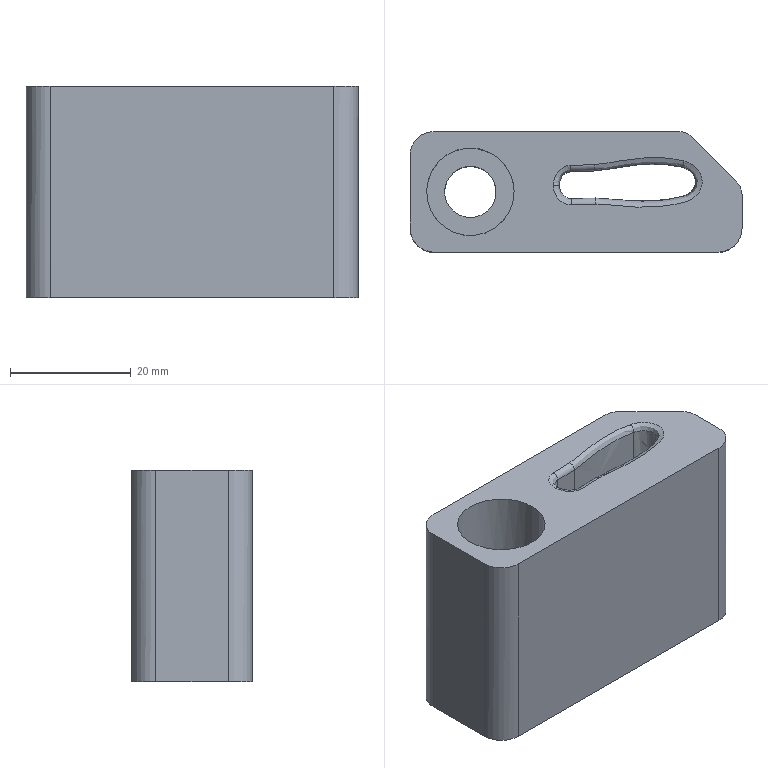Part | NX | features DIE-6 2 | 1 solid | 35 faces | box 55 x 20 x 35 mm | volume 29138 mm3 | plane 16 | cylinder 11 | spline 8 | commonest cylinder face diameters 8 x3 2 x2 5 x2 6 x2 8.506 x1 14.5 x1